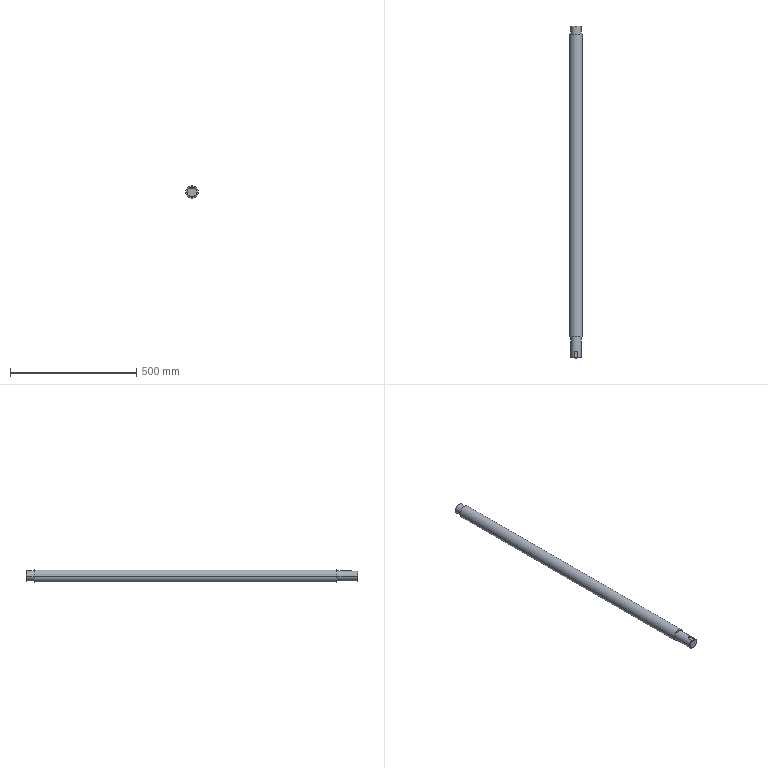Part | SolidWorks | features ICE 2, BaseBody 1, Chamfer 1 | 1 solid | 19 faces | box 50 x 1316 x 50 mm | volume 2500128 mm3 | cylinder 7 | plane 7 | cone 5 | commonest cylinder face diameters 40 x4 50 x2 12 x1
STEP:
#1=CARTESIAN_POINT('',(18.,-683.649,0.));
#2=VERTEX_POINT('',#1);
#3=CARTESIAN_POINT('',(6.,-683.649,16.971));
#4=VERTEX_POINT('',#3);
#5=CARTESIAN_POINT('',(0.,-683.649,0.));
#6=DIRECTION('',(0.,-1.,0.));
#7=DIRECTION('',(1.,0.,0.));
#8=AXIS2_PLACEMENT_3D('',#5,#6,#7);
#9=CIRCLE('',#8,18.);
#10=EDGE_CURVE('',#2,#4,#9,.T.);
#11=ORIENTED_EDGE('',*,*,#10,.F.);
#12=CARTESIAN_POINT('',(20.,-681.649,0.));
#13=VERTEX_POINT('',#12);
#14=CARTESIAN_POINT('',(20.,-681.649,0.));
#15=DIRECTION('',(0.7071,0.7071,0.));
#16=VECTOR('',#15,1000.);
#17=LINE('',#14,#16);
#18=EDGE_CURVE('',#2,#13,#17,.T.);
#19=ORIENTED_EDGE('',*,*,#18,.T.);
#20=CARTESIAN_POINT('',(6.,-681.649,19.079));
#21=VERTEX_POINT('',#20);
#22=CARTESIAN_POINT('',(0.,-681.649,0.));
#23=DIRECTION('',(0.,1.,0.));
#24=DIRECTION('',(1.,0.,0.));
#25=AXIS2_PLACEMENT_3D('',#22,#23,#24);
#26=CIRCLE('',#25,20.);
#27=EDGE_CURVE('',#21,#13,#26,.T.);
#28=ORIENTED_EDGE('',*,*,#27,.F.);
#29=CARTESIAN_POINT('',(6.,-683.649,16.971));
#30=CARTESIAN_POINT('',(6.,-682.984,17.675));
#31=CARTESIAN_POINT('',(6.,-682.317,18.378));
#32=CARTESIAN_POINT('',(6.,-681.649,19.079));
#33=B_SPLINE_CURVE_WITH_KNOTS('',3,(#29,#30,#31,#32),.UNSPECIFIED.,.F.,.F.,(4,4),(0.,0.002906),.UNSPECIFIED.);
#34=EDGE_CURVE('',#4,#21,#33,.T.);
#35=ORIENTED_EDGE('',*,*,#34,.F.);
#36=EDGE_LOOP('',(#11,#19,#28,#35));
#37=FACE_OUTER_BOUND('',#36,.T.);
#38=CARTESIAN_POINT('',(0.,-681.649,0.));
#39=DIRECTION('',(0.,1.,0.));
#40=DIRECTION('',(-1.,0.,0.));
#41=AXIS2_PLACEMENT_3D('',#38,#39,#40);
#42=CONICAL_SURFACE('',#41,20.,0.7854);
#43=ADVANCED_FACE('',(#37),#42,.T.);
#44=ORIENTED_EDGE('',*,*,#18,.F.);
#45=CARTESIAN_POINT('',(-18.,-683.649,0.));
#46=VERTEX_POINT('',#45);
#47=CARTESIAN_POINT('',(0.,-683.649,0.));
#48=DIRECTION('',(0.,-1.,0.));
#49=DIRECTION('',(1.,0.,0.));
#50=AXIS2_PLACEMENT_3D('',#47,#48,#49);
#51=CIRCLE('',#50,18.);
#52=EDGE_CURVE('',#46,#2,#51,.T.);
#53=ORIENTED_EDGE('',*,*,#52,.F.);
#54=CARTESIAN_POINT('',(-20.,-681.649,0.));
#55=VERTEX_POINT('',#54);
#56=CARTESIAN_POINT('',(-20.,-681.649,0.));
#57=DIRECTION('',(-0.7071,0.7071,0.));
#58=VECTOR('',#57,1000.);
#59=LINE('',#56,#58);
#60=EDGE_CURVE('',#46,#55,#59,.T.);
#61=ORIENTED_EDGE('',*,*,#60,.T.);
#62=CARTESIAN_POINT('',(0.,-681.649,0.));
#63=DIRECTION('',(0.,1.,0.));
#64=DIRECTION('',(1.,0.,0.));
#65=AXIS2_PLACEMENT_3D('',#62,#63,#64);
#66=CIRCLE('',#65,20.);
#67=EDGE_CURVE('',#13,#55,#66,.T.);
#68=ORIENTED_EDGE('',*,*,#67,.F.);
#69=EDGE_LOOP('',(#44,#53,#61,#68));
#70=FACE_OUTER_BOUND('',#69,.T.);
#71=CARTESIAN_POINT('',(0.,-681.649,0.));
#72=DIRECTION('',(0.,1.,0.));
#73=DIRECTION('',(-1.,0.,0.));
#74=AXIS2_PLACEMENT_3D('',#71,#72,#73);
#75=CONICAL_SURFACE('',#74,20.,0.7854);
#76=ADVANCED_FACE('',(#70),#75,.T.);
#77=CARTESIAN_POINT('',(-18.,632.369,0.));
#78=VERTEX_POINT('',#77);
#79=CARTESIAN_POINT('',(18.,632.369,0.));
#80=VERTEX_POINT('',#79);
#81=CARTESIAN_POINT('',(0.,632.369,0.));
#82=DIRECTION('',(0.,1.,0.));
#83=DIRECTION('',(-1.,0.,0.));
#84=AXIS2_PLACEMENT_3D('',#81,#82,#83);
#85=CIRCLE('',#84,18.);
#86=EDGE_CURVE('',#78,#80,#85,.T.);
#87=ORIENTED_EDGE('',*,*,#86,.F.);
#88=CARTESIAN_POINT('',(-20.,630.369,0.));
#89=VERTEX_POINT('',#88);
#90=CARTESIAN_POINT('',(-20.,630.369,0.));
#91=DIRECTION('',(-0.7071,-0.7071,0.));
#92=VECTOR('',#91,1000.);
#93=LINE('',#90,#92);
#94=EDGE_CURVE('',#78,#89,#93,.T.);
#95=ORIENTED_EDGE('',*,*,#94,.T.);
#96=CARTESIAN_POINT('',(20.,630.369,0.));
#97=VERTEX_POINT('',#96);
#98=CARTESIAN_POINT('',(0.,630.369,0.));
#99=DIRECTION('',(0.,-1.,0.));
#100=DIRECTION('',(-1.,0.,0.));
#101=AXIS2_PLACEMENT_3D('',#98,#99,#100);
#102=CIRCLE('',#101,20.);
#103=EDGE_CURVE('',#97,#89,#102,.T.);
#104=ORIENTED_EDGE('',*,*,#103,.F.);
#105=CARTESIAN_POINT('',(20.,630.369,0.));
#106=DIRECTION('',(0.7071,-0.7071,0.));
#107=VECTOR('',#106,1000.);
#108=LINE('',#105,#107);
#109=EDGE_CURVE('',#80,#97,#108,.T.);
#110=ORIENTED_EDGE('',*,*,#109,.F.);
#111=EDGE_LOOP('',(#87,#95,#104,#110));
#112=FACE_OUTER_BOUND('',#111,.T.);
#113=CARTESIAN_POINT('',(0.,630.369,0.));
#114=DIRECTION('',(0.,-1.,0.));
#115=DIRECTION('',(1.,0.,0.));
#116=AXIS2_PLACEMENT_3D('',#113,#114,#115);
#117=CONICAL_SURFACE('',#116,20.,0.7854);
#118=ADVANCED_FACE('',(#112),#117,.T.);
#119=CARTESIAN_POINT('',(25.,600.,0.));
#120=VERTEX_POINT('',#119);
#121=CARTESIAN_POINT('',(-25.,600.,0.));
#122=VERTEX_POINT('',#121);
#123=CARTESIAN_POINT('',(0.,600.,0.));
#124=DIRECTION('',(0.,-1.,0.));
#125=DIRECTION('',(1.,0.,0.));
#126=AXIS2_PLACEMENT_3D('',#123,#124,#125);
#127=CIRCLE('',#126,25.);
#128=EDGE_CURVE('',#120,#122,#127,.T.);
#129=ORIENTED_EDGE('',*,*,#128,.T.);
#130=CARTESIAN_POINT('',(-25.,-600.,0.));
#131=VERTEX_POINT('',#130);
#132=CARTESIAN_POINT('',(-25.,0.,0.));
#133=DIRECTION('',(0.,-1.,0.));
#134=VECTOR('',#133,1000.);
#135=LINE('',#132,#134);
#136=EDGE_CURVE('',#122,#131,#135,.T.);
#137=ORIENTED_EDGE('',*,*,#136,.T.);
#138=CARTESIAN_POINT('',(25.,-600.,0.));
#139=VERTEX_POINT('',#138);
#140=CARTESIAN_POINT('',(0.,-600.,0.));
#141=DIRECTION('',(0.,1.,0.));
#142=DIRECTION('',(1.,0.,0.));
#143=AXIS2_PLACEMENT_3D('',#140,#141,#142);
#144=CIRCLE('',#143,25.);
#145=EDGE_CURVE('',#131,#139,#144,.T.);
#146=ORIENTED_EDGE('',*,*,#145,.T.);
#147=CARTESIAN_POINT('',(25.,0.,0.));
#148=DIRECTION('',(0.,-1.,0.));
#149=VECTOR('',#148,1000.);
#150=LINE('',#147,#149);
#151=EDGE_CURVE('',#120,#139,#150,.T.);
#152=ORIENTED_EDGE('',*,*,#151,.F.);
#153=EDGE_LOOP('',(#129,#137,#146,#152));
#154=FACE_OUTER_BOUND('',#153,.T.);
#155=CARTESIAN_POINT('',(0.,0.,0.));
#156=DIRECTION('',(0.,-1.,0.));
#157=DIRECTION('',(1.,0.,0.));
#158=AXIS2_PLACEMENT_3D('',#155,#156,#157);
#159=CYLINDRICAL_SURFACE('',#158,25.);
#160=ADVANCED_FACE('',(#154),#159,.T.);
#161=ORIENTED_EDGE('',*,*,#103,.T.);
#162=CARTESIAN_POINT('',(-20.,600.,0.));
#163=VERTEX_POINT('',#162);
#164=CARTESIAN_POINT('',(-20.,616.185,0.));
#165=DIRECTION('',(0.,-1.,0.));
#166=VECTOR('',#165,1000.);
#167=LINE('',#164,#166);
#168=EDGE_CURVE('',#89,#163,#167,.T.);
#169=ORIENTED_EDGE('',*,*,#168,.T.);
#170=CARTESIAN_POINT('',(20.,600.,0.));
#171=VERTEX_POINT('',#170);
#172=CARTESIAN_POINT('',(0.,600.,0.));
#173=DIRECTION('',(0.,-1.,0.));
#174=DIRECTION('',(1.,0.,0.));
#175=AXIS2_PLACEMENT_3D('',#172,#173,#174);
#176=CIRCLE('',#175,20.);
#177=EDGE_CURVE('',#171,#163,#176,.T.);
#178=ORIENTED_EDGE('',*,*,#177,.F.);
#179=CARTESIAN_POINT('',(20.,616.185,0.));
#180=DIRECTION('',(0.,-1.,0.));
#181=VECTOR('',#180,1000.);
#182=LINE('',#179,#181);
#183=EDGE_CURVE('',#97,#171,#182,.T.);
#184=ORIENTED_EDGE('',*,*,#183,.F.);
#185=EDGE_LOOP('',(#161,#169,#178,#184));
#186=FACE_OUTER_BOUND('',#185,.T.);
#187=CARTESIAN_POINT('',(0.,616.185,0.));
#188=DIRECTION('',(0.,-1.,0.));
#189=DIRECTION('',(1.,0.,0.));
#190=AXIS2_PLACEMENT_3D('',#187,#188,#189);
#191=CYLINDRICAL_SURFACE('',#190,20.);
#192=ADVANCED_FACE('',(#186),#191,.T.);
#193=CARTESIAN_POINT('',(-20.,-600.,0.));
#194=VERTEX_POINT('',#193);
#195=CARTESIAN_POINT('',(20.,-600.,0.));
#196=VERTEX_POINT('',#195);
#197=CARTESIAN_POINT('',(0.,-600.,0.));
#198=DIRECTION('',(0.,1.,0.));
#199=DIRECTION('',(1.,0.,0.));
#200=AXIS2_PLACEMENT_3D('',#197,#198,#199);
#201=CIRCLE('',#200,20.);
#202=EDGE_CURVE('',#194,#196,#201,.T.);
#203=ORIENTED_EDGE('',*,*,#202,.F.);
#204=CARTESIAN_POINT('',(-20.,-641.824,0.));
#205=DIRECTION('',(0.,-1.,0.));
#206=VECTOR('',#205,1000.);
#207=LINE('',#204,#206);
#208=EDGE_CURVE('',#194,#55,#207,.T.);
#209=ORIENTED_EDGE('',*,*,#208,.T.);
#210=CARTESIAN_POINT('',(-6.,-681.649,19.079));
#211=VERTEX_POINT('',#210);
#212=CARTESIAN_POINT('',(0.,-681.649,0.));
#213=DIRECTION('',(0.,1.,0.));
#214=DIRECTION('',(1.,0.,0.));
#215=AXIS2_PLACEMENT_3D('',#212,#213,#214);
#216=CIRCLE('',#215,20.);
#217=EDGE_CURVE('',#55,#211,#216,.T.);
#218=ORIENTED_EDGE('',*,*,#217,.T.);
#219=CARTESIAN_POINT('',(-6.,-663.649,19.079));
#220=VERTEX_POINT('',#219);
#221=CARTESIAN_POINT('',(-6.,-641.824,19.079));
#222=DIRECTION('',(0.,-1.,0.));
#223=VECTOR('',#222,1000.);
#224=LINE('',#221,#223);
#225=EDGE_CURVE('',#220,#211,#224,.T.);
#226=ORIENTED_EDGE('',*,*,#225,.F.);
#227=CARTESIAN_POINT('',(6.,-663.649,19.079));
#228=VERTEX_POINT('',#227);
#229=CARTESIAN_POINT('',(-6.,-663.649,19.079));
#230=CARTESIAN_POINT('',(-6.,-663.25,19.079));
#231=CARTESIAN_POINT('',(-5.961,-662.858,19.091));
#232=CARTESIAN_POINT('',(-5.845,-662.28,19.127));
#233=CARTESIAN_POINT('',(-5.797,-662.09,19.141));
#234=CARTESIAN_POINT('',(-5.682,-661.711,19.176));
#235=CARTESIAN_POINT('',(-5.615,-661.524,19.196));
#236=CARTESIAN_POINT('',(-5.388,-660.98,19.261));
#237=CARTESIAN_POINT('',(-5.204,-660.636,19.312));
#238=CARTESIAN_POINT('',(-4.877,-660.149,19.396));
#239=CARTESIAN_POINT('',(-4.759,-659.99,19.426));
#240=CARTESIAN_POINT('',(-4.51,-659.687,19.485));
#241=CARTESIAN_POINT('',(-4.379,-659.543,19.515));
#242=CARTESIAN_POINT('',(-3.967,-659.13,19.605));
#243=CARTESIAN_POINT('',(-3.666,-658.882,19.664));
#244=CARTESIAN_POINT('',(-3.011,-658.444,19.775));
#245=CARTESIAN_POINT('',(-2.665,-658.259,19.825));
#246=CARTESIAN_POINT('',(-2.124,-658.034,19.888));
#247=CARTESIAN_POINT('',(-1.94,-657.967,19.907));
#248=CARTESIAN_POINT('',(-1.563,-657.852,19.94));
#249=CARTESIAN_POINT('',(-1.369,-657.804,19.954));
#250=CARTESIAN_POINT('',(-0.7875,-657.687,19.988));
#251=CARTESIAN_POINT('',(-0.3966,-657.649,20.));
#252=CARTESIAN_POINT('',(0.3914,-657.648,20.));
#253=CARTESIAN_POINT('',(0.7916,-657.688,19.988));
#254=CARTESIAN_POINT('',(1.563,-657.842,19.943));
#255=CARTESIAN_POINT('',(1.938,-657.957,19.909));
#256=CARTESIAN_POINT('',(2.668,-658.26,19.825));
#257=CARTESIAN_POINT('',(3.015,-658.447,19.774));
#258=CARTESIAN_POINT('',(3.501,-658.772,19.692));
#259=CARTESIAN_POINT('',(3.657,-658.888,19.663));
#260=CARTESIAN_POINT('',(3.96,-659.137,19.605));
#261=CARTESIAN_POINT('',(4.106,-659.27,19.574));
#262=CARTESIAN_POINT('',(4.522,-659.685,19.484));
#263=CARTESIAN_POINT('',(4.768,-659.986,19.425));
#264=CARTESIAN_POINT('',(5.202,-660.634,19.313));
#265=CARTESIAN_POINT('',(5.391,-660.985,19.26));
#266=CARTESIAN_POINT('',(5.691,-661.708,19.174));
#267=CARTESIAN_POINT('',(5.805,-662.082,19.139));
#268=CARTESIAN_POINT('',(5.922,-662.664,19.103));
#269=CARTESIAN_POINT('',(5.951,-662.862,19.094));
#270=CARTESIAN_POINT('',(5.99,-663.255,19.082));
#271=CARTESIAN_POINT('',(6.,-663.452,19.079));
#272=CARTESIAN_POINT('',(6.,-663.649,19.079));
#273=B_SPLINE_CURVE_WITH_KNOTS('',3,(#229,#230,#231,#232,#233,#234,#235,#236,#237,#238,#239,#240,#241,#242,#243,#244,#245,#246,#247,#248,#249,#250,#251,#252,#253,#254,#255,#256,#257,#258,#259,#260,#261,#262,#263,#264,#265,#266,#267,#268,#269,#270,#271,#272),.UNSPECIFIED.,.F.,.F.,(4,2,2,2,2,2,2,2,2,2,2,2,2,2,2,2,2,2,2,2,2,4),(0.,0.001179,0.001769,0.002358,0.003538,0.004127,0.004717,0.005896,0.007075,0.007665,0.008255,0.009434,0.01061,0.01179,0.01297,0.01356,0.01415,0.01533,0.01651,0.01769,0.01828,0.01887),.UNSPECIFIED.);
#274=EDGE_CURVE('',#220,#228,#273,.T.);
#275=ORIENTED_EDGE('',*,*,#274,.T.);
#276=CARTESIAN_POINT('',(6.,-641.824,19.079));
#277=DIRECTION('',(0.,1.,0.));
#278=VECTOR('',#277,1000.);
#279=LINE('',#276,#278);
#280=EDGE_CURVE('',#21,#228,#279,.T.);
#281=ORIENTED_EDGE('',*,*,#280,.F.);
#282=ORIENTED_EDGE('',*,*,#27,.T.);
#283=CARTESIAN_POINT('',(20.,-641.824,0.));
#284=DIRECTION('',(0.,-1.,0.));
#285=VECTOR('',#284,1000.);
#286=LINE('',#283,#285);
#287=EDGE_CURVE('',#196,#13,#286,.T.);
#288=ORIENTED_EDGE('',*,*,#287,.F.);
#289=EDGE_LOOP('',(#203,#209,#218,#226,#275,#281,#282,#288));
#290=FACE_OUTER_BOUND('',#289,.T.);
#291=CARTESIAN_POINT('',(0.,-641.824,0.));
#292=DIRECTION('',(0.,-1.,0.));
#293=DIRECTION('',(1.,0.,0.));
#294=AXIS2_PLACEMENT_3D('',#291,#292,#293);
#295=CYLINDRICAL_SURFACE('',#294,20.);
#296=ADVANCED_FACE('',(#290),#295,.T.);
#297=ORIENTED_EDGE('',*,*,#208,.F.);
#298=CARTESIAN_POINT('',(0.,-600.,0.));
#299=DIRECTION('',(0.,1.,0.));
#300=DIRECTION('',(1.,0.,0.));
#301=AXIS2_PLACEMENT_3D('',#298,#299,#300);
#302=CIRCLE('',#301,20.);
#303=EDGE_CURVE('',#196,#194,#302,.T.);
#304=ORIENTED_EDGE('',*,*,#303,.F.);
#305=ORIENTED_EDGE('',*,*,#287,.T.);
#306=ORIENTED_EDGE('',*,*,#67,.T.);
#307=EDGE_LOOP('',(#297,#304,#305,#306));
#308=FACE_OUTER_BOUND('',#307,.T.);
#309=CARTESIAN_POINT('',(0.,-641.824,0.));
#310=DIRECTION('',(0.,-1.,0.));
#311=DIRECTION('',(1.,0.,0.));
#312=AXIS2_PLACEMENT_3D('',#309,#310,#311);
#313=CYLINDRICAL_SURFACE('',#312,20.);
#314=ADVANCED_FACE('',(#308),#313,.T.);
#315=ORIENTED_EDGE('',*,*,#136,.F.);
#316=CARTESIAN_POINT('',(0.,600.,0.));
#317=DIRECTION('',(0.,-1.,0.));
#318=DIRECTION('',(1.,0.,0.));
#319=AXIS2_PLACEMENT_3D('',#316,#317,#318);
#320=CIRCLE('',#319,25.);
#321=EDGE_CURVE('',#122,#120,#320,.T.);
#322=ORIENTED_EDGE('',*,*,#321,.T.);
#323=ORIENTED_EDGE('',*,*,#151,.T.);
#324=CARTESIAN_POINT('',(0.,-600.,0.));
#325=DIRECTION('',(0.,1.,0.));
#326=DIRECTION('',(1.,0.,0.));
#327=AXIS2_PLACEMENT_3D('',#324,#325,#326);
#328=CIRCLE('',#327,25.);
#329=EDGE_CURVE('',#139,#131,#328,.T.);
#330=ORIENTED_EDGE('',*,*,#329,.T.);
#331=EDGE_LOOP('',(#315,#322,#323,#330));
#332=FACE_OUTER_BOUND('',#331,.T.);
#333=CARTESIAN_POINT('',(0.,0.,0.));
#334=DIRECTION('',(0.,-1.,0.));
#335=DIRECTION('',(1.,0.,0.));
#336=AXIS2_PLACEMENT_3D('',#333,#334,#335);
#337=CYLINDRICAL_SURFACE('',#336,25.);
#338=ADVANCED_FACE('',(#332),#337,.T.);
#339=ORIENTED_EDGE('',*,*,#177,.T.);
#340=CARTESIAN_POINT('',(0.,600.,0.));
#341=DIRECTION('',(0.,-1.,0.));
#342=DIRECTION('',(1.,0.,0.));
#343=AXIS2_PLACEMENT_3D('',#340,#341,#342);
#344=CIRCLE('',#343,20.);
#345=EDGE_CURVE('',#163,#171,#344,.T.);
#346=ORIENTED_EDGE('',*,*,#345,.T.);
#347=EDGE_LOOP('',(#339,#346));
#348=FACE_BOUND('',#347,.T.);
#349=ORIENTED_EDGE('',*,*,#128,.F.);
#350=ORIENTED_EDGE('',*,*,#321,.F.);
#351=EDGE_LOOP('',(#349,#350));
#352=FACE_OUTER_BOUND('',#351,.T.);
#353=CARTESIAN_POINT('',(25.,600.,0.));
#354=DIRECTION('',(0.,1.,0.));
#355=DIRECTION('',(-1.,0.,0.));
#356=AXIS2_PLACEMENT_3D('',#353,#354,#355);
#357=PLANE('',#356);
#358=ADVANCED_FACE('',(#348,#352),#357,.T.);
#359=ORIENTED_EDGE('',*,*,#303,.T.);
#360=ORIENTED_EDGE('',*,*,#202,.T.);
#361=EDGE_LOOP('',(#359,#360));
#362=FACE_BOUND('',#361,.T.);
#363=ORIENTED_EDGE('',*,*,#329,.F.);
#364=ORIENTED_EDGE('',*,*,#145,.F.);
#365=EDGE_LOOP('',(#363,#364));
#366=FACE_OUTER_BOUND('',#365,.T.);
#367=CARTESIAN_POINT('',(20.,-600.,0.));
#368=DIRECTION('',(0.,-1.,0.));
#369=DIRECTION('',(1.,0.,0.));
#370=AXIS2_PLACEMENT_3D('',#367,#368,#369);
#371=PLANE('',#370);
#372=ADVANCED_FACE('',(#362,#366),#371,.T.);
#373=ORIENTED_EDGE('',*,*,#168,.F.);
#374=CARTESIAN_POINT('',(0.,630.369,0.));
#375=DIRECTION('',(0.,-1.,0.));
#376=DIRECTION('',(-1.,0.,0.));
#377=AXIS2_PLACEMENT_3D('',#374,#375,#376);
#378=CIRCLE('',#377,20.);
#379=EDGE_CURVE('',#89,#97,#378,.T.);
#380=ORIENTED_EDGE('',*,*,#379,.T.);
#381=ORIENTED_EDGE('',*,*,#183,.T.);
#382=ORIENTED_EDGE('',*,*,#345,.F.);
#383=EDGE_LOOP('',(#373,#380,#381,#382));
#384=FACE_OUTER_BOUND('',#383,.T.);
#385=CARTESIAN_POINT('',(0.,616.185,0.));
#386=DIRECTION('',(0.,-1.,0.));
#387=DIRECTION('',(1.,0.,0.));
#388=AXIS2_PLACEMENT_3D('',#385,#386,#387);
#389=CYLINDRICAL_SURFACE('',#388,20.);
#390=ADVANCED_FACE('',(#384),#389,.T.);
#391=CARTESIAN_POINT('',(0.,632.369,0.));
#392=DIRECTION('',(0.,1.,0.));
#393=DIRECTION('',(-1.,0.,0.));
#394=AXIS2_PLACEMENT_3D('',#391,#392,#393);
#395=CIRCLE('',#394,18.);
#396=EDGE_CURVE('',#80,#78,#395,.T.);
#397=ORIENTED_EDGE('',*,*,#396,.T.);
#398=ORIENTED_EDGE('',*,*,#86,.T.);
#399=EDGE_LOOP('',(#397,#398));
#400=FACE_OUTER_BOUND('',#399,.T.);
#401=CARTESIAN_POINT('',(20.,632.369,0.));
#402=DIRECTION('',(0.,1.,0.));
#403=DIRECTION('',(-1.,0.,0.));
#404=AXIS2_PLACEMENT_3D('',#401,#402,#403);
#405=PLANE('',#404);
#406=ADVANCED_FACE('',(#400),#405,.T.);
#407=CARTESIAN_POINT('',(-6.,-683.649,16.971));
#408=VERTEX_POINT('',#407);
#409=CARTESIAN_POINT('',(-6.,-683.649,15.));
#410=VERTEX_POINT('',#409);
#411=CARTESIAN_POINT('',(-6.,-683.649,20.));
#412=DIRECTION('',(0.,0.,-1.));
#413=VECTOR('',#412,1000.);
#414=LINE('',#411,#413);
#415=EDGE_CURVE('',#408,#410,#414,.T.);
#416=ORIENTED_EDGE('',*,*,#415,.F.);
#417=CARTESIAN_POINT('',(0.,-683.649,0.));
#418=DIRECTION('',(0.,-1.,0.));
#419=DIRECTION('',(1.,0.,0.));
#420=AXIS2_PLACEMENT_3D('',#417,#418,#419);
#421=CIRCLE('',#420,18.);
#422=EDGE_CURVE('',#408,#46,#421,.T.);
#423=ORIENTED_EDGE('',*,*,#422,.T.);
#424=ORIENTED_EDGE('',*,*,#52,.T.);
#425=ORIENTED_EDGE('',*,*,#10,.T.);
#426=CARTESIAN_POINT('',(6.,-683.649,15.));
#427=VERTEX_POINT('',#426);
#428=CARTESIAN_POINT('',(6.,-683.649,20.));
#429=DIRECTION('',(0.,0.,1.));
#430=VECTOR('',#429,1000.);
#431=LINE('',#428,#430);
#432=EDGE_CURVE('',#427,#4,#431,.T.);
#433=ORIENTED_EDGE('',*,*,#432,.F.);
#434=CARTESIAN_POINT('',(-6.,-683.649,15.));
#435=DIRECTION('',(1.,0.,0.));
#436=VECTOR('',#435,1000.);
#437=LINE('',#434,#436);
#438=EDGE_CURVE('',#410,#427,#437,.T.);
#439=ORIENTED_EDGE('',*,*,#438,.F.);
#440=EDGE_LOOP('',(#416,#423,#424,#425,#433,#439));
#441=FACE_OUTER_BOUND('',#440,.T.);
#442=CARTESIAN_POINT('',(0.,-683.649,0.));
#443=DIRECTION('',(0.,-1.,0.));
#444=DIRECTION('',(1.,0.,0.));
#445=AXIS2_PLACEMENT_3D('',#442,#443,#444);
#446=PLANE('',#445);
#447=ADVANCED_FACE('',(#441),#446,.T.);
#448=ORIENTED_EDGE('',*,*,#225,.T.);
#449=CARTESIAN_POINT('',(-6.,-681.649,19.079));
#450=CARTESIAN_POINT('',(-6.,-682.317,18.378));
#451=CARTESIAN_POINT('',(-6.,-682.984,17.675));
#452=CARTESIAN_POINT('',(-6.,-683.649,16.971));
#453=B_SPLINE_CURVE_WITH_KNOTS('',3,(#449,#450,#451,#452),.UNSPECIFIED.,.F.,.F.,(4,4),(0.,0.002906),.UNSPECIFIED.);
#454=EDGE_CURVE('',#211,#408,#453,.T.);
#455=ORIENTED_EDGE('',*,*,#454,.T.);
#456=ORIENTED_EDGE('',*,*,#415,.T.);
#457=CARTESIAN_POINT('',(-6.,-663.649,15.));
#458=VERTEX_POINT('',#457);
#459=CARTESIAN_POINT('',(-6.,-663.649,15.));
#460=DIRECTION('',(0.,-1.,0.));
#461=VECTOR('',#460,1000.);
#462=LINE('',#459,#461);
#463=EDGE_CURVE('',#458,#410,#462,.T.);
#464=ORIENTED_EDGE('',*,*,#463,.F.);
#465=CARTESIAN_POINT('',(-6.,-663.649,20.));
#466=DIRECTION('',(0.,0.,-1.));
#467=VECTOR('',#466,1000.);
#468=LINE('',#465,#467);
#469=EDGE_CURVE('',#220,#458,#468,.T.);
#470=ORIENTED_EDGE('',*,*,#469,.F.);
#471=EDGE_LOOP('',(#448,#455,#456,#464,#470));
#472=FACE_OUTER_BOUND('',#471,.T.);
#473=CARTESIAN_POINT('',(-6.,-663.649,20.));
#474=DIRECTION('',(-1.,0.,0.));
#475=DIRECTION('',(0.,-1.,0.));
#476=AXIS2_PLACEMENT_3D('',#473,#474,#475);
#477=PLANE('',#476);
#478=ADVANCED_FACE('',(#472),#477,.F.);
#479=ORIENTED_EDGE('',*,*,#432,.T.);
#480=ORIENTED_EDGE('',*,*,#34,.T.);
#481=ORIENTED_EDGE('',*,*,#280,.T.);
#482=CARTESIAN_POINT('',(6.,-663.649,15.));
#483=VERTEX_POINT('',#482);
#484=CARTESIAN_POINT('',(6.,-663.649,20.));
#485=DIRECTION('',(0.,0.,1.));
#486=VECTOR('',#485,1000.);
#487=LINE('',#484,#486);
#488=EDGE_CURVE('',#483,#228,#487,.T.);
#489=ORIENTED_EDGE('',*,*,#488,.F.);
#490=CARTESIAN_POINT('',(6.,-663.649,15.));
#491=DIRECTION('',(0.,-1.,0.));
#492=VECTOR('',#491,1000.);
#493=LINE('',#490,#492);
#494=EDGE_CURVE('',#483,#427,#493,.T.);
#495=ORIENTED_EDGE('',*,*,#494,.T.);
#496=EDGE_LOOP('',(#479,#480,#481,#489,#495));
#497=FACE_OUTER_BOUND('',#496,.T.);
#498=CARTESIAN_POINT('',(6.,-663.649,20.));
#499=DIRECTION('',(1.,0.,0.));
#500=DIRECTION('',(0.,1.,0.));
#501=AXIS2_PLACEMENT_3D('',#498,#499,#500);
#502=PLANE('',#501);
#503=ADVANCED_FACE('',(#497),#502,.F.);
#504=ORIENTED_EDGE('',*,*,#494,.F.);
#505=CARTESIAN_POINT('',(0.,-663.649,15.));
#506=DIRECTION('',(0.,0.,1.));
#507=DIRECTION('',(1.,0.,0.));
#508=AXIS2_PLACEMENT_3D('',#505,#506,#507);
#509=CIRCLE('',#508,6.);
#510=EDGE_CURVE('',#483,#458,#509,.T.);
#511=ORIENTED_EDGE('',*,*,#510,.T.);
#512=ORIENTED_EDGE('',*,*,#463,.T.);
#513=ORIENTED_EDGE('',*,*,#438,.T.);
#514=EDGE_LOOP('',(#504,#511,#512,#513));
#515=FACE_OUTER_BOUND('',#514,.T.);
#516=CARTESIAN_POINT('',(-6.,-663.649,15.));
#517=DIRECTION('',(0.,0.,-1.));
#518=DIRECTION('',(-1.,0.,0.));
#519=AXIS2_PLACEMENT_3D('',#516,#517,#518);
#520=PLANE('',#519);
#521=ADVANCED_FACE('',(#515),#520,.F.);
#522=ORIENTED_EDGE('',*,*,#510,.F.);
#523=ORIENTED_EDGE('',*,*,#488,.T.);
#524=ORIENTED_EDGE('',*,*,#274,.F.);
#525=ORIENTED_EDGE('',*,*,#469,.T.);
#526=EDGE_LOOP('',(#522,#523,#524,#525));
#527=FACE_OUTER_BOUND('',#526,.T.);
#528=CARTESIAN_POINT('',(0.,-663.649,25.));
#529=DIRECTION('',(0.,0.,-1.));
#530=DIRECTION('',(-1.,0.,0.));
#531=AXIS2_PLACEMENT_3D('',#528,#529,#530);
#532=CYLINDRICAL_SURFACE('',#531,6.);
#533=ADVANCED_FACE('',(#527),#532,.F.);
#534=ORIENTED_EDGE('',*,*,#94,.F.);
#535=ORIENTED_EDGE('',*,*,#396,.F.);
#536=ORIENTED_EDGE('',*,*,#109,.T.);
#537=ORIENTED_EDGE('',*,*,#379,.F.);
#538=EDGE_LOOP('',(#534,#535,#536,#537));
#539=FACE_OUTER_BOUND('',#538,.T.);
#540=CARTESIAN_POINT('',(0.,630.369,0.));
#541=DIRECTION('',(0.,-1.,0.));
#542=DIRECTION('',(1.,0.,0.));
#543=AXIS2_PLACEMENT_3D('',#540,#541,#542);
#544=CONICAL_SURFACE('',#543,20.,0.7854);
#545=ADVANCED_FACE('',(#539),#544,.T.);
#546=ORIENTED_EDGE('',*,*,#60,.F.);
#547=ORIENTED_EDGE('',*,*,#422,.F.);
#548=ORIENTED_EDGE('',*,*,#454,.F.);
#549=ORIENTED_EDGE('',*,*,#217,.F.);
#550=EDGE_LOOP('',(#546,#547,#548,#549));
#551=FACE_OUTER_BOUND('',#550,.T.);
#552=CARTESIAN_POINT('',(0.,-681.649,0.));
#553=DIRECTION('',(0.,1.,0.));
#554=DIRECTION('',(-1.,0.,0.));
#555=AXIS2_PLACEMENT_3D('',#552,#553,#554);
#556=CONICAL_SURFACE('',#555,20.,0.7854);
#557=ADVANCED_FACE('',(#551),#556,.T.);
#558=CLOSED_SHELL('',(#43,#76,#118,#160,#192,#296,#314,#338,#358,#372,#390,#406,#447,#478,#503,#521,#533,#545,#557));
#559=MANIFOLD_SOLID_BREP('',#558);
#560=CARTESIAN_POINT('',(0.,0.,0.));
#561=DIRECTION('',(0.,0.,1.));
#562=DIRECTION('',(1.,0.,0.));
#563=AXIS2_PLACEMENT_3D('',#560,#561,#562);
#564=(LENGTH_UNIT()NAMED_UNIT(*)SI_UNIT(.MILLI.,.METRE.));
#565=UNCERTAINTY_MEASURE_WITH_UNIT(LENGTH_MEASURE(0.00001),#564,'','');
#566=(NAMED_UNIT(*)PLANE_ANGLE_UNIT()SI_UNIT($,.RADIAN.));
#567=(NAMED_UNIT(*)SI_UNIT($,.STERADIAN.)SOLID_ANGLE_UNIT());
#568=(GEOMETRIC_REPRESENTATION_CONTEXT(3)GLOBAL_UNCERTAINTY_ASSIGNED_CONTEXT((#565))GLOBAL_UNIT_ASSIGNED_CONTEXT((#564,#566,#567))REPRESENTATION_CONTEXT('',''));
#569=ADVANCED_BREP_SHAPE_REPRESENTATION('',(#559,#563),#568);